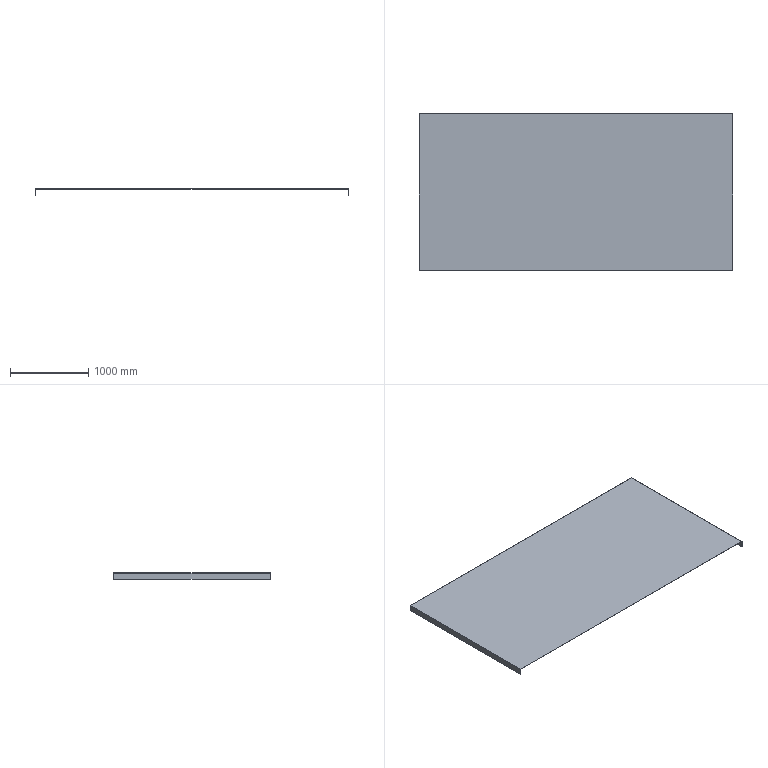Part | SolidWorks | features ICE 2, Extrusion 1 | 1 solid | 10 faces | box 4008 x 2000 x 80 mm | volume 16656000 mm3 | plane 10
STEP:
#1=CARTESIAN_POINT('',(2002.,1000.,0.));
#2=VERTEX_POINT('',#1);
#3=CARTESIAN_POINT('',(-2002.,1000.,0.));
#4=VERTEX_POINT('',#3);
#5=CARTESIAN_POINT('',(-2002.,1000.,0.));
#6=DIRECTION('',(-1.,0.,0.));
#7=VECTOR('',#6,1000.);
#8=LINE('',#5,#7);
#9=EDGE_CURVE('',#2,#4,#8,.T.);
#10=ORIENTED_EDGE('',*,*,#9,.T.);
#11=CARTESIAN_POINT('',(-2002.,1000.,-78.));
#12=VERTEX_POINT('',#11);
#13=CARTESIAN_POINT('',(-2002.,1000.,2.));
#14=DIRECTION('',(0.,0.,-1.));
#15=VECTOR('',#14,1000.);
#16=LINE('',#13,#15);
#17=EDGE_CURVE('',#4,#12,#16,.T.);
#18=ORIENTED_EDGE('',*,*,#17,.T.);
#19=CARTESIAN_POINT('',(-2004.,1000.,-78.));
#20=VERTEX_POINT('',#19);
#21=CARTESIAN_POINT('',(-2004.,1000.,-78.));
#22=DIRECTION('',(1.,0.,0.));
#23=VECTOR('',#22,1000.);
#24=LINE('',#21,#23);
#25=EDGE_CURVE('',#20,#12,#24,.T.);
#26=ORIENTED_EDGE('',*,*,#25,.F.);
#27=CARTESIAN_POINT('',(-2004.,1000.,2.));
#28=VERTEX_POINT('',#27);
#29=CARTESIAN_POINT('',(-2004.,1000.,2.));
#30=DIRECTION('',(0.,0.,-1.));
#31=VECTOR('',#30,1000.);
#32=LINE('',#29,#31);
#33=EDGE_CURVE('',#28,#20,#32,.T.);
#34=ORIENTED_EDGE('',*,*,#33,.F.);
#35=CARTESIAN_POINT('',(2004.,1000.,2.));
#36=VERTEX_POINT('',#35);
#37=CARTESIAN_POINT('',(-2002.,1000.,2.));
#38=DIRECTION('',(-1.,0.,0.));
#39=VECTOR('',#38,1000.);
#40=LINE('',#37,#39);
#41=EDGE_CURVE('',#36,#28,#40,.T.);
#42=ORIENTED_EDGE('',*,*,#41,.F.);
#43=CARTESIAN_POINT('',(2004.,1000.,-78.));
#44=VERTEX_POINT('',#43);
#45=CARTESIAN_POINT('',(2004.,1000.,-78.));
#46=DIRECTION('',(0.,0.,1.));
#47=VECTOR('',#46,1000.);
#48=LINE('',#45,#47);
#49=EDGE_CURVE('',#44,#36,#48,.T.);
#50=ORIENTED_EDGE('',*,*,#49,.F.);
#51=CARTESIAN_POINT('',(2002.,1000.,-78.));
#52=VERTEX_POINT('',#51);
#53=CARTESIAN_POINT('',(2004.,1000.,-78.));
#54=DIRECTION('',(-1.,0.,0.));
#55=VECTOR('',#54,1000.);
#56=LINE('',#53,#55);
#57=EDGE_CURVE('',#44,#52,#56,.T.);
#58=ORIENTED_EDGE('',*,*,#57,.T.);
#59=CARTESIAN_POINT('',(2002.,1000.,-78.));
#60=DIRECTION('',(0.,0.,1.));
#61=VECTOR('',#60,1000.);
#62=LINE('',#59,#61);
#63=EDGE_CURVE('',#52,#2,#62,.T.);
#64=ORIENTED_EDGE('',*,*,#63,.T.);
#65=EDGE_LOOP('',(#10,#18,#26,#34,#42,#50,#58,#64));
#66=FACE_OUTER_BOUND('',#65,.T.);
#67=CARTESIAN_POINT('',(-2002.,1000.,2.));
#68=DIRECTION('',(0.,-1.,0.));
#69=DIRECTION('',(0.,0.,-1.));
#70=AXIS2_PLACEMENT_3D('',#67,#68,#69);
#71=PLANE('',#70);
#72=ADVANCED_FACE('',(#66),#71,.F.);
#73=CARTESIAN_POINT('',(-2002.,-1000.,0.));
#74=VERTEX_POINT('',#73);
#75=CARTESIAN_POINT('',(2002.,-1000.,0.));
#76=VERTEX_POINT('',#75);
#77=CARTESIAN_POINT('',(-2002.,-1000.,0.));
#78=DIRECTION('',(1.,0.,0.));
#79=VECTOR('',#78,1000.);
#80=LINE('',#77,#79);
#81=EDGE_CURVE('',#74,#76,#80,.T.);
#82=ORIENTED_EDGE('',*,*,#81,.T.);
#83=CARTESIAN_POINT('',(2002.,-1000.,-78.));
#84=VERTEX_POINT('',#83);
#85=CARTESIAN_POINT('',(2002.,-1000.,2.));
#86=DIRECTION('',(0.,0.,-1.));
#87=VECTOR('',#86,1000.);
#88=LINE('',#85,#87);
#89=EDGE_CURVE('',#76,#84,#88,.T.);
#90=ORIENTED_EDGE('',*,*,#89,.T.);
#91=CARTESIAN_POINT('',(2004.,-1000.,-78.));
#92=VERTEX_POINT('',#91);
#93=CARTESIAN_POINT('',(2004.,-1000.,-78.));
#94=DIRECTION('',(-1.,0.,0.));
#95=VECTOR('',#94,1000.);
#96=LINE('',#93,#95);
#97=EDGE_CURVE('',#92,#84,#96,.T.);
#98=ORIENTED_EDGE('',*,*,#97,.F.);
#99=CARTESIAN_POINT('',(2004.,-1000.,2.));
#100=VERTEX_POINT('',#99);
#101=CARTESIAN_POINT('',(2004.,-1000.,2.));
#102=DIRECTION('',(0.,0.,-1.));
#103=VECTOR('',#102,1000.);
#104=LINE('',#101,#103);
#105=EDGE_CURVE('',#100,#92,#104,.T.);
#106=ORIENTED_EDGE('',*,*,#105,.F.);
#107=CARTESIAN_POINT('',(-2004.,-1000.,2.));
#108=VERTEX_POINT('',#107);
#109=CARTESIAN_POINT('',(-2002.,-1000.,2.));
#110=DIRECTION('',(1.,0.,0.));
#111=VECTOR('',#110,1000.);
#112=LINE('',#109,#111);
#113=EDGE_CURVE('',#108,#100,#112,.T.);
#114=ORIENTED_EDGE('',*,*,#113,.F.);
#115=CARTESIAN_POINT('',(-2004.,-1000.,-78.));
#116=VERTEX_POINT('',#115);
#117=CARTESIAN_POINT('',(-2004.,-1000.,2.));
#118=DIRECTION('',(0.,0.,1.));
#119=VECTOR('',#118,1000.);
#120=LINE('',#117,#119);
#121=EDGE_CURVE('',#116,#108,#120,.T.);
#122=ORIENTED_EDGE('',*,*,#121,.F.);
#123=CARTESIAN_POINT('',(-2002.,-1000.,-78.));
#124=VERTEX_POINT('',#123);
#125=CARTESIAN_POINT('',(-2004.,-1000.,-78.));
#126=DIRECTION('',(1.,0.,0.));
#127=VECTOR('',#126,1000.);
#128=LINE('',#125,#127);
#129=EDGE_CURVE('',#116,#124,#128,.T.);
#130=ORIENTED_EDGE('',*,*,#129,.T.);
#131=CARTESIAN_POINT('',(-2002.,-1000.,2.));
#132=DIRECTION('',(0.,0.,1.));
#133=VECTOR('',#132,1000.);
#134=LINE('',#131,#133);
#135=EDGE_CURVE('',#124,#74,#134,.T.);
#136=ORIENTED_EDGE('',*,*,#135,.T.);
#137=EDGE_LOOP('',(#82,#90,#98,#106,#114,#122,#130,#136));
#138=FACE_OUTER_BOUND('',#137,.T.);
#139=CARTESIAN_POINT('',(-2002.,-1000.,2.));
#140=DIRECTION('',(0.,1.,0.));
#141=DIRECTION('',(0.,0.,1.));
#142=AXIS2_PLACEMENT_3D('',#139,#140,#141);
#143=PLANE('',#142);
#144=ADVANCED_FACE('',(#138),#143,.F.);
#145=ORIENTED_EDGE('',*,*,#113,.T.);
#146=CARTESIAN_POINT('',(2004.,1000.,2.));
#147=DIRECTION('',(0.,-1.,0.));
#148=VECTOR('',#147,1000.);
#149=LINE('',#146,#148);
#150=EDGE_CURVE('',#36,#100,#149,.T.);
#151=ORIENTED_EDGE('',*,*,#150,.F.);
#152=ORIENTED_EDGE('',*,*,#41,.T.);
#153=CARTESIAN_POINT('',(-2004.,1000.,2.));
#154=DIRECTION('',(0.,1.,0.));
#155=VECTOR('',#154,1000.);
#156=LINE('',#153,#155);
#157=EDGE_CURVE('',#108,#28,#156,.T.);
#158=ORIENTED_EDGE('',*,*,#157,.F.);
#159=EDGE_LOOP('',(#145,#151,#152,#158));
#160=FACE_OUTER_BOUND('',#159,.T.);
#161=CARTESIAN_POINT('',(0.,0.,2.));
#162=DIRECTION('',(0.,0.,1.));
#163=DIRECTION('',(1.,0.,0.));
#164=AXIS2_PLACEMENT_3D('',#161,#162,#163);
#165=PLANE('',#164);
#166=ADVANCED_FACE('',(#160),#165,.T.);
#167=CARTESIAN_POINT('',(2002.,1000.,0.));
#168=DIRECTION('',(0.,1.,0.));
#169=VECTOR('',#168,1000.);
#170=LINE('',#167,#169);
#171=EDGE_CURVE('',#76,#2,#170,.T.);
#172=ORIENTED_EDGE('',*,*,#171,.F.);
#173=ORIENTED_EDGE('',*,*,#81,.F.);
#174=CARTESIAN_POINT('',(-2002.,1000.,0.));
#175=DIRECTION('',(0.,-1.,0.));
#176=VECTOR('',#175,1000.);
#177=LINE('',#174,#176);
#178=EDGE_CURVE('',#4,#74,#177,.T.);
#179=ORIENTED_EDGE('',*,*,#178,.F.);
#180=ORIENTED_EDGE('',*,*,#9,.F.);
#181=EDGE_LOOP('',(#172,#173,#179,#180));
#182=FACE_OUTER_BOUND('',#181,.T.);
#183=CARTESIAN_POINT('',(0.,0.,0.));
#184=DIRECTION('',(0.,0.,1.));
#185=DIRECTION('',(1.,0.,0.));
#186=AXIS2_PLACEMENT_3D('',#183,#184,#185);
#187=PLANE('',#186);
#188=ADVANCED_FACE('',(#182),#187,.F.);
#189=CARTESIAN_POINT('',(-2002.,1000.,-78.));
#190=DIRECTION('',(0.,-1.,0.));
#191=VECTOR('',#190,1000.);
#192=LINE('',#189,#191);
#193=EDGE_CURVE('',#12,#124,#192,.T.);
#194=ORIENTED_EDGE('',*,*,#193,.T.);
#195=ORIENTED_EDGE('',*,*,#129,.F.);
#196=CARTESIAN_POINT('',(-2004.,1000.,-78.));
#197=DIRECTION('',(0.,-1.,0.));
#198=VECTOR('',#197,1000.);
#199=LINE('',#196,#198);
#200=EDGE_CURVE('',#20,#116,#199,.T.);
#201=ORIENTED_EDGE('',*,*,#200,.F.);
#202=ORIENTED_EDGE('',*,*,#25,.T.);
#203=EDGE_LOOP('',(#194,#195,#201,#202));
#204=FACE_OUTER_BOUND('',#203,.T.);
#205=CARTESIAN_POINT('',(-2004.,1000.,-78.));
#206=DIRECTION('',(0.,0.,1.));
#207=DIRECTION('',(0.,-1.,0.));
#208=AXIS2_PLACEMENT_3D('',#205,#206,#207);
#209=PLANE('',#208);
#210=ADVANCED_FACE('',(#204),#209,.F.);
#211=ORIENTED_EDGE('',*,*,#157,.T.);
#212=ORIENTED_EDGE('',*,*,#33,.T.);
#213=ORIENTED_EDGE('',*,*,#200,.T.);
#214=ORIENTED_EDGE('',*,*,#121,.T.);
#215=EDGE_LOOP('',(#211,#212,#213,#214));
#216=FACE_OUTER_BOUND('',#215,.T.);
#217=CARTESIAN_POINT('',(-2004.,0.,0.));
#218=DIRECTION('',(1.,0.,0.));
#219=DIRECTION('',(0.,1.,0.));
#220=AXIS2_PLACEMENT_3D('',#217,#218,#219);
#221=PLANE('',#220);
#222=ADVANCED_FACE('',(#216),#221,.F.);
#223=ORIENTED_EDGE('',*,*,#17,.F.);
#224=ORIENTED_EDGE('',*,*,#178,.T.);
#225=ORIENTED_EDGE('',*,*,#135,.F.);
#226=ORIENTED_EDGE('',*,*,#193,.F.);
#227=EDGE_LOOP('',(#223,#224,#225,#226));
#228=FACE_OUTER_BOUND('',#227,.T.);
#229=CARTESIAN_POINT('',(-2002.,0.,0.));
#230=DIRECTION('',(1.,0.,0.));
#231=DIRECTION('',(0.,1.,0.));
#232=AXIS2_PLACEMENT_3D('',#229,#230,#231);
#233=PLANE('',#232);
#234=ADVANCED_FACE('',(#228),#233,.T.);
#235=ORIENTED_EDGE('',*,*,#89,.F.);
#236=ORIENTED_EDGE('',*,*,#171,.T.);
#237=ORIENTED_EDGE('',*,*,#63,.F.);
#238=CARTESIAN_POINT('',(2002.,-1000.,-78.));
#239=DIRECTION('',(0.,1.,0.));
#240=VECTOR('',#239,1000.);
#241=LINE('',#238,#240);
#242=EDGE_CURVE('',#84,#52,#241,.T.);
#243=ORIENTED_EDGE('',*,*,#242,.F.);
#244=EDGE_LOOP('',(#235,#236,#237,#243));
#245=FACE_OUTER_BOUND('',#244,.T.);
#246=CARTESIAN_POINT('',(2002.,0.,0.));
#247=DIRECTION('',(1.,0.,0.));
#248=DIRECTION('',(0.,0.,-1.));
#249=AXIS2_PLACEMENT_3D('',#246,#247,#248);
#250=PLANE('',#249);
#251=ADVANCED_FACE('',(#245),#250,.F.);
#252=ORIENTED_EDGE('',*,*,#242,.T.);
#253=ORIENTED_EDGE('',*,*,#57,.F.);
#254=CARTESIAN_POINT('',(2004.,-1000.,-78.));
#255=DIRECTION('',(0.,1.,0.));
#256=VECTOR('',#255,1000.);
#257=LINE('',#254,#256);
#258=EDGE_CURVE('',#92,#44,#257,.T.);
#259=ORIENTED_EDGE('',*,*,#258,.F.);
#260=ORIENTED_EDGE('',*,*,#97,.T.);
#261=EDGE_LOOP('',(#252,#253,#259,#260));
#262=FACE_OUTER_BOUND('',#261,.T.);
#263=CARTESIAN_POINT('',(2004.,-1000.,-78.));
#264=DIRECTION('',(0.,0.,1.));
#265=DIRECTION('',(0.,-1.,0.));
#266=AXIS2_PLACEMENT_3D('',#263,#264,#265);
#267=PLANE('',#266);
#268=ADVANCED_FACE('',(#262),#267,.F.);
#269=ORIENTED_EDGE('',*,*,#150,.T.);
#270=ORIENTED_EDGE('',*,*,#105,.T.);
#271=ORIENTED_EDGE('',*,*,#258,.T.);
#272=ORIENTED_EDGE('',*,*,#49,.T.);
#273=EDGE_LOOP('',(#269,#270,#271,#272));
#274=FACE_OUTER_BOUND('',#273,.T.);
#275=CARTESIAN_POINT('',(2004.,0.,0.));
#276=DIRECTION('',(1.,0.,0.));
#277=DIRECTION('',(0.,0.,-1.));
#278=AXIS2_PLACEMENT_3D('',#275,#276,#277);
#279=PLANE('',#278);
#280=ADVANCED_FACE('',(#274),#279,.T.);
#281=CLOSED_SHELL('',(#72,#144,#166,#188,#210,#222,#234,#251,#268,#280));
#282=MANIFOLD_SOLID_BREP('',#281);
#283=CARTESIAN_POINT('',(0.,0.,0.));
#284=DIRECTION('',(0.,0.,1.));
#285=DIRECTION('',(1.,0.,0.));
#286=AXIS2_PLACEMENT_3D('',#283,#284,#285);
#287=(LENGTH_UNIT()NAMED_UNIT(*)SI_UNIT(.MILLI.,.METRE.));
#288=UNCERTAINTY_MEASURE_WITH_UNIT(LENGTH_MEASURE(0.00001),#287,'','');
#289=(NAMED_UNIT(*)PLANE_ANGLE_UNIT()SI_UNIT($,.RADIAN.));
#290=(NAMED_UNIT(*)SI_UNIT($,.STERADIAN.)SOLID_ANGLE_UNIT());
#291=(GEOMETRIC_REPRESENTATION_CONTEXT(3)GLOBAL_UNCERTAINTY_ASSIGNED_CONTEXT((#288))GLOBAL_UNIT_ASSIGNED_CONTEXT((#287,#289,#290))REPRESENTATION_CONTEXT('',''));
#292=ADVANCED_BREP_SHAPE_REPRESENTATION('',(#282,#286),#291);